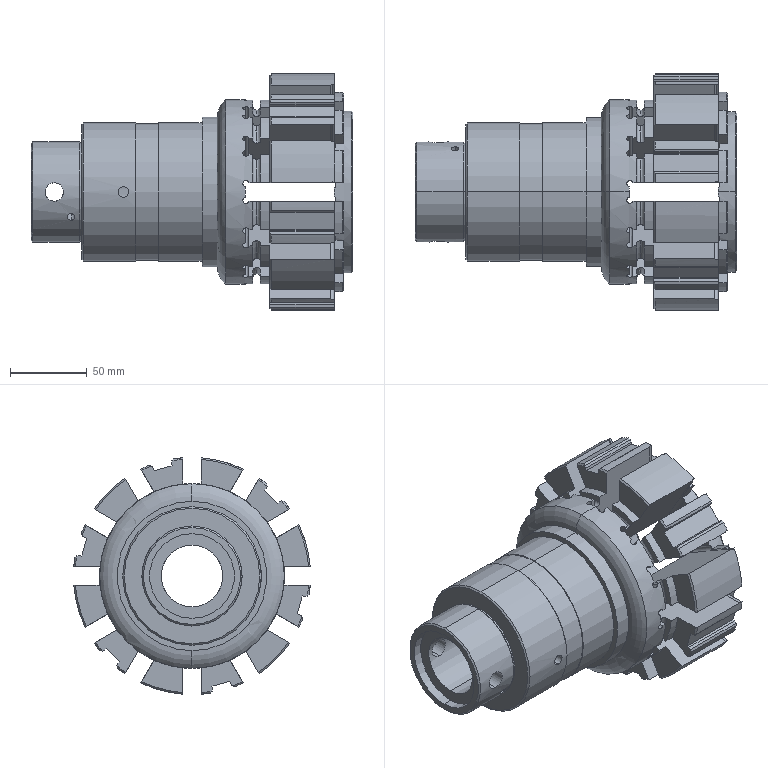Part | SolidWorks | features ICE 9, 3DProfileFeature 6, CirPattern 6, HoleWzd 6, Chamfer 2, RefAxis 1, RevCut 1, Revolution 1 | 1 solid | 396 faces | box 209 x 153.532 x 153.532 mm | volume 1079981 mm3 | plane 184 | cylinder 148 | cone 38 | torus 26 | commonest cylinder face diameters 4 x72 154 x18 120 x14 130 x12 5 x4 12 x4